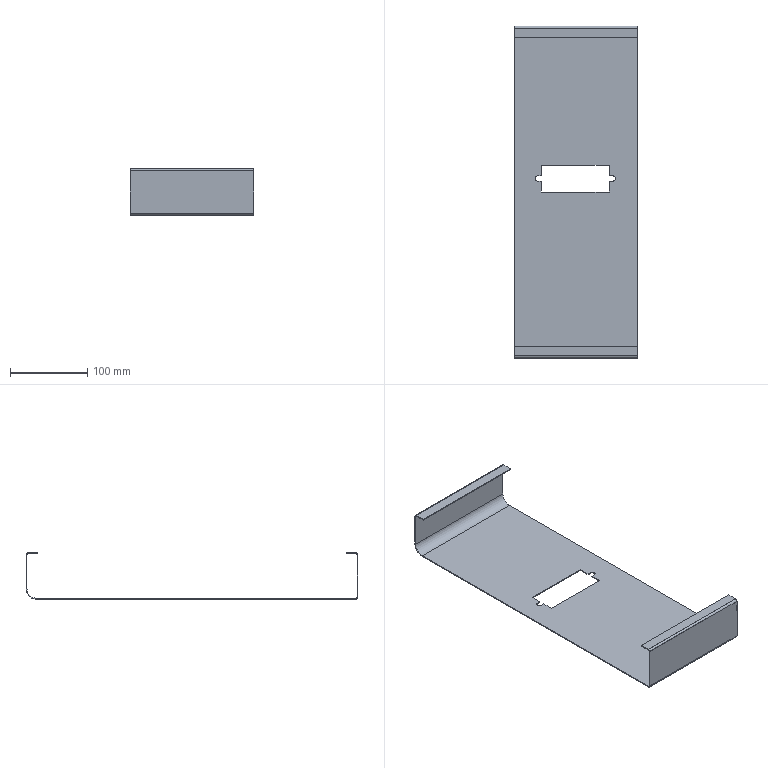Part | SolidWorks | features FlatPattern 1, ICE 1, SMBaseFlange 1, SheetMetal 1 | 1 solid | 51 faces | box 160 x 430 x 60 mm | volume 105063 mm3 | plane 40 | cylinder 11 | commonest cylinder face diameters 3 x3 5.4 x3 7 x3 24 x1 26.4 x1
STEP:
#1=CARTESIAN_POINT('',(-49.5,21.,1.2));
#2=VERTEX_POINT('',#1);
#3=CARTESIAN_POINT('',(-53.,17.5,1.2));
#4=VERTEX_POINT('',#3);
#5=CARTESIAN_POINT('',(-49.5,17.5,1.2));
#6=DIRECTION('',(0.,0.,1.));
#7=DIRECTION('',(0.,1.,0.));
#8=AXIS2_PLACEMENT_3D('',#5,#6,#7);
#9=CIRCLE('',#8,3.5);
#10=EDGE_CURVE('',#2,#4,#9,.T.);
#11=ORIENTED_EDGE('',*,*,#10,.T.);
#12=CARTESIAN_POINT('',(-53.,17.5,0.));
#13=VERTEX_POINT('',#12);
#14=CARTESIAN_POINT('',(-53.,17.5,60.001));
#15=DIRECTION('',(0.,0.,-1.));
#16=VECTOR('',#15,1000.);
#17=LINE('',#14,#16);
#18=EDGE_CURVE('',#4,#13,#17,.T.);
#19=ORIENTED_EDGE('',*,*,#18,.T.);
#20=CARTESIAN_POINT('',(-49.5,21.,0.));
#21=VERTEX_POINT('',#20);
#22=CARTESIAN_POINT('',(-49.5,17.5,0.));
#23=DIRECTION('',(0.,0.,-1.));
#24=DIRECTION('',(-1.,0.,0.));
#25=AXIS2_PLACEMENT_3D('',#22,#23,#24);
#26=CIRCLE('',#25,3.5);
#27=EDGE_CURVE('',#13,#21,#26,.T.);
#28=ORIENTED_EDGE('',*,*,#27,.T.);
#29=CARTESIAN_POINT('',(-49.5,21.,60.001));
#30=DIRECTION('',(0.,0.,-1.));
#31=VECTOR('',#30,1000.);
#32=LINE('',#29,#31);
#33=EDGE_CURVE('',#2,#21,#32,.T.);
#34=ORIENTED_EDGE('',*,*,#33,.F.);
#35=EDGE_LOOP('',(#11,#19,#28,#34));
#36=FACE_OUTER_BOUND('',#35,.T.);
#37=CARTESIAN_POINT('',(-49.5,17.5,60.001));
#38=DIRECTION('',(0.,0.,-1.));
#39=DIRECTION('',(-1.,0.,0.));
#40=AXIS2_PLACEMENT_3D('',#37,#38,#39);
#41=CYLINDRICAL_SURFACE('',#40,3.5);
#42=ADVANCED_FACE('',(#36),#41,.F.);
#43=CARTESIAN_POINT('',(80.,201.8,0.));
#44=VERTEX_POINT('',#43);
#45=CARTESIAN_POINT('',(80.,201.8,1.2));
#46=VERTEX_POINT('',#45);
#47=CARTESIAN_POINT('',(80.,201.8,0.));
#48=DIRECTION('',(0.,0.,1.));
#49=VECTOR('',#48,1000.);
#50=LINE('',#47,#49);
#51=EDGE_CURVE('',#44,#46,#50,.T.);
#52=ORIENTED_EDGE('',*,*,#51,.F.);
#53=CARTESIAN_POINT('',(80.,215.,13.2));
#54=VERTEX_POINT('',#53);
#55=CARTESIAN_POINT('',(80.,201.8,13.2));
#56=DIRECTION('',(-1.,0.,0.));
#57=DIRECTION('',(0.,0.,-1.));
#58=AXIS2_PLACEMENT_3D('',#55,#56,#57);
#59=CIRCLE('',#58,13.2);
#60=EDGE_CURVE('',#54,#44,#59,.T.);
#61=ORIENTED_EDGE('',*,*,#60,.F.);
#62=CARTESIAN_POINT('',(80.,213.8,13.2));
#63=VERTEX_POINT('',#62);
#64=CARTESIAN_POINT('',(80.,213.8,13.2));
#65=DIRECTION('',(0.,1.,0.));
#66=VECTOR('',#65,1000.);
#67=LINE('',#64,#66);
#68=EDGE_CURVE('',#63,#54,#67,.T.);
#69=ORIENTED_EDGE('',*,*,#68,.F.);
#70=CARTESIAN_POINT('',(80.,201.8,13.2));
#71=DIRECTION('',(-1.,0.,0.));
#72=DIRECTION('',(0.,0.,-1.));
#73=AXIS2_PLACEMENT_3D('',#70,#71,#72);
#74=CIRCLE('',#73,12.);
#75=EDGE_CURVE('',#63,#46,#74,.T.);
#76=ORIENTED_EDGE('',*,*,#75,.T.);
#77=EDGE_LOOP('',(#52,#61,#69,#76));
#78=FACE_OUTER_BOUND('',#77,.T.);
#79=CARTESIAN_POINT('',(80.,201.8,0.));
#80=DIRECTION('',(1.,0.,0.));
#81=DIRECTION('',(0.,0.,-1.));
#82=AXIS2_PLACEMENT_3D('',#79,#80,#81);
#83=PLANE('',#82);
#84=ADVANCED_FACE('',(#78),#83,.T.);
#85=CARTESIAN_POINT('',(80.,-212.3,0.));
#86=VERTEX_POINT('',#85);
#87=CARTESIAN_POINT('',(80.,0.,0.));
#88=DIRECTION('',(0.,-1.,0.));
#89=VECTOR('',#88,1000.);
#90=LINE('',#87,#89);
#91=EDGE_CURVE('',#44,#86,#90,.T.);
#92=ORIENTED_EDGE('',*,*,#91,.F.);
#93=ORIENTED_EDGE('',*,*,#51,.T.);
#94=CARTESIAN_POINT('',(80.,-212.3,1.2));
#95=VERTEX_POINT('',#94);
#96=CARTESIAN_POINT('',(80.,0.,1.2));
#97=DIRECTION('',(0.,-1.,0.));
#98=VECTOR('',#97,1000.);
#99=LINE('',#96,#98);
#100=EDGE_CURVE('',#46,#95,#99,.T.);
#101=ORIENTED_EDGE('',*,*,#100,.T.);
#102=CARTESIAN_POINT('',(80.,-212.3,1.2));
#103=DIRECTION('',(0.,0.,-1.));
#104=VECTOR('',#103,1000.);
#105=LINE('',#102,#104);
#106=EDGE_CURVE('',#95,#86,#105,.T.);
#107=ORIENTED_EDGE('',*,*,#106,.T.);
#108=EDGE_LOOP('',(#92,#93,#101,#107));
#109=FACE_OUTER_BOUND('',#108,.T.);
#110=CARTESIAN_POINT('',(80.,213.8,13.2));
#111=DIRECTION('',(1.,0.,0.));
#112=DIRECTION('',(0.,0.,-1.));
#113=AXIS2_PLACEMENT_3D('',#110,#111,#112);
#114=PLANE('',#113);
#115=ADVANCED_FACE('',(#109),#114,.T.);
#116=CARTESIAN_POINT('',(-80.,215.,13.2));
#117=VERTEX_POINT('',#116);
#118=CARTESIAN_POINT('',(-80.,213.8,13.2));
#119=VERTEX_POINT('',#118);
#120=CARTESIAN_POINT('',(-80.,215.,13.2));
#121=DIRECTION('',(0.,-1.,0.));
#122=VECTOR('',#121,1000.);
#123=LINE('',#120,#122);
#124=EDGE_CURVE('',#117,#119,#123,.T.);
#125=ORIENTED_EDGE('',*,*,#124,.F.);
#126=CARTESIAN_POINT('',(-80.,201.8,0.));
#127=VERTEX_POINT('',#126);
#128=CARTESIAN_POINT('',(-80.,201.8,13.2));
#129=DIRECTION('',(-1.,0.,0.));
#130=DIRECTION('',(0.,0.,-1.));
#131=AXIS2_PLACEMENT_3D('',#128,#129,#130);
#132=CIRCLE('',#131,13.2);
#133=EDGE_CURVE('',#117,#127,#132,.T.);
#134=ORIENTED_EDGE('',*,*,#133,.T.);
#135=CARTESIAN_POINT('',(-80.,201.8,1.2));
#136=VERTEX_POINT('',#135);
#137=CARTESIAN_POINT('',(-80.,201.8,1.2));
#138=DIRECTION('',(0.,0.,-1.));
#139=VECTOR('',#138,1000.);
#140=LINE('',#137,#139);
#141=EDGE_CURVE('',#136,#127,#140,.T.);
#142=ORIENTED_EDGE('',*,*,#141,.F.);
#143=CARTESIAN_POINT('',(-80.,201.8,13.2));
#144=DIRECTION('',(-1.,0.,0.));
#145=DIRECTION('',(0.,0.,-1.));
#146=AXIS2_PLACEMENT_3D('',#143,#144,#145);
#147=CIRCLE('',#146,12.);
#148=EDGE_CURVE('',#119,#136,#147,.T.);
#149=ORIENTED_EDGE('',*,*,#148,.F.);
#150=EDGE_LOOP('',(#125,#134,#142,#149));
#151=FACE_OUTER_BOUND('',#150,.T.);
#152=CARTESIAN_POINT('',(-80.,215.,13.2));
#153=DIRECTION('',(-1.,0.,0.));
#154=DIRECTION('',(0.,0.,1.));
#155=AXIS2_PLACEMENT_3D('',#152,#153,#154);
#156=PLANE('',#155);
#157=ADVANCED_FACE('',(#151),#156,.T.);
#158=CARTESIAN_POINT('',(-80.,215.,57.3));
#159=VERTEX_POINT('',#158);
#160=CARTESIAN_POINT('',(-80.,215.,13.2));
#161=DIRECTION('',(0.,0.,-1.));
#162=VECTOR('',#161,1000.);
#163=LINE('',#160,#162);
#164=EDGE_CURVE('',#159,#117,#163,.T.);
#165=ORIENTED_EDGE('',*,*,#164,.T.);
#166=ORIENTED_EDGE('',*,*,#124,.T.);
#167=CARTESIAN_POINT('',(-80.,213.8,57.3));
#168=VERTEX_POINT('',#167);
#169=CARTESIAN_POINT('',(-80.,213.8,13.2));
#170=DIRECTION('',(0.,0.,-1.));
#171=VECTOR('',#170,1000.);
#172=LINE('',#169,#171);
#173=EDGE_CURVE('',#168,#119,#172,.T.);
#174=ORIENTED_EDGE('',*,*,#173,.F.);
#175=CARTESIAN_POINT('',(-80.,213.8,57.3));
#176=DIRECTION('',(0.,1.,0.));
#177=VECTOR('',#176,1000.);
#178=LINE('',#175,#177);
#179=EDGE_CURVE('',#168,#159,#178,.T.);
#180=ORIENTED_EDGE('',*,*,#179,.T.);
#181=EDGE_LOOP('',(#165,#166,#174,#180));
#182=FACE_OUTER_BOUND('',#181,.T.);
#183=CARTESIAN_POINT('',(-80.,201.8,1.2));
#184=DIRECTION('',(-1.,0.,0.));
#185=DIRECTION('',(0.,0.,1.));
#186=AXIS2_PLACEMENT_3D('',#183,#184,#185);
#187=PLANE('',#186);
#188=ADVANCED_FACE('',(#182),#187,.T.);
#189=CARTESIAN_POINT('',(80.,215.,57.3));
#190=VERTEX_POINT('',#189);
#191=CARTESIAN_POINT('',(80.,213.8,57.3));
#192=VERTEX_POINT('',#191);
#193=CARTESIAN_POINT('',(80.,215.,57.3));
#194=DIRECTION('',(0.,-1.,0.));
#195=VECTOR('',#194,1000.);
#196=LINE('',#193,#195);
#197=EDGE_CURVE('',#190,#192,#196,.T.);
#198=ORIENTED_EDGE('',*,*,#197,.F.);
#199=CARTESIAN_POINT('',(80.,212.3,60.));
#200=VERTEX_POINT('',#199);
#201=CARTESIAN_POINT('',(80.,212.3,57.3));
#202=DIRECTION('',(-1.,0.,0.));
#203=DIRECTION('',(0.,0.,-1.));
#204=AXIS2_PLACEMENT_3D('',#201,#202,#203);
#205=CIRCLE('',#204,2.7);
#206=EDGE_CURVE('',#200,#190,#205,.T.);
#207=ORIENTED_EDGE('',*,*,#206,.F.);
#208=CARTESIAN_POINT('',(80.,212.3,58.8));
#209=VERTEX_POINT('',#208);
#210=CARTESIAN_POINT('',(80.,212.3,58.8));
#211=DIRECTION('',(0.,0.,1.));
#212=VECTOR('',#211,1000.);
#213=LINE('',#210,#212);
#214=EDGE_CURVE('',#209,#200,#213,.T.);
#215=ORIENTED_EDGE('',*,*,#214,.F.);
#216=CARTESIAN_POINT('',(80.,212.3,57.3));
#217=DIRECTION('',(-1.,0.,0.));
#218=DIRECTION('',(0.,0.,-1.));
#219=AXIS2_PLACEMENT_3D('',#216,#217,#218);
#220=CIRCLE('',#219,1.5);
#221=EDGE_CURVE('',#209,#192,#220,.T.);
#222=ORIENTED_EDGE('',*,*,#221,.T.);
#223=EDGE_LOOP('',(#198,#207,#215,#222));
#224=FACE_OUTER_BOUND('',#223,.T.);
#225=CARTESIAN_POINT('',(80.,215.,57.3));
#226=DIRECTION('',(1.,0.,0.));
#227=DIRECTION('',(0.,0.,-1.));
#228=AXIS2_PLACEMENT_3D('',#225,#226,#227);
#229=PLANE('',#228);
#230=ADVANCED_FACE('',(#224),#229,.T.);
#231=CARTESIAN_POINT('',(80.,215.,13.2));
#232=DIRECTION('',(0.,0.,-1.));
#233=VECTOR('',#232,1000.);
#234=LINE('',#231,#233);
#235=EDGE_CURVE('',#190,#54,#234,.T.);
#236=ORIENTED_EDGE('',*,*,#235,.F.);
#237=ORIENTED_EDGE('',*,*,#197,.T.);
#238=CARTESIAN_POINT('',(80.,213.8,13.2));
#239=DIRECTION('',(0.,0.,-1.));
#240=VECTOR('',#239,1000.);
#241=LINE('',#238,#240);
#242=EDGE_CURVE('',#192,#63,#241,.T.);
#243=ORIENTED_EDGE('',*,*,#242,.T.);
#244=ORIENTED_EDGE('',*,*,#68,.T.);
#245=EDGE_LOOP('',(#236,#237,#243,#244));
#246=FACE_OUTER_BOUND('',#245,.T.);
#247=CARTESIAN_POINT('',(80.,212.3,58.8));
#248=DIRECTION('',(1.,0.,0.));
#249=DIRECTION('',(0.,0.,-1.));
#250=AXIS2_PLACEMENT_3D('',#247,#248,#249);
#251=PLANE('',#250);
#252=ADVANCED_FACE('',(#246),#251,.T.);
#253=CARTESIAN_POINT('',(-80.,212.3,60.));
#254=VERTEX_POINT('',#253);
#255=CARTESIAN_POINT('',(-80.,212.3,58.8));
#256=VERTEX_POINT('',#255);
#257=CARTESIAN_POINT('',(-80.,212.3,60.));
#258=DIRECTION('',(0.,0.,-1.));
#259=VECTOR('',#258,1000.);
#260=LINE('',#257,#259);
#261=EDGE_CURVE('',#254,#256,#260,.T.);
#262=ORIENTED_EDGE('',*,*,#261,.F.);
#263=CARTESIAN_POINT('',(-80.,212.3,57.3));
#264=DIRECTION('',(-1.,0.,0.));
#265=DIRECTION('',(0.,0.,-1.));
#266=AXIS2_PLACEMENT_3D('',#263,#264,#265);
#267=CIRCLE('',#266,2.7);
#268=EDGE_CURVE('',#254,#159,#267,.T.);
#269=ORIENTED_EDGE('',*,*,#268,.T.);
#270=ORIENTED_EDGE('',*,*,#179,.F.);
#271=CARTESIAN_POINT('',(-80.,212.3,57.3));
#272=DIRECTION('',(-1.,0.,0.));
#273=DIRECTION('',(0.,0.,-1.));
#274=AXIS2_PLACEMENT_3D('',#271,#272,#273);
#275=CIRCLE('',#274,1.5);
#276=EDGE_CURVE('',#256,#168,#275,.T.);
#277=ORIENTED_EDGE('',*,*,#276,.F.);
#278=EDGE_LOOP('',(#262,#269,#270,#277));
#279=FACE_OUTER_BOUND('',#278,.T.);
#280=CARTESIAN_POINT('',(-80.,212.3,60.));
#281=DIRECTION('',(-1.,0.,0.));
#282=DIRECTION('',(0.,0.,1.));
#283=AXIS2_PLACEMENT_3D('',#280,#281,#282);
#284=PLANE('',#283);
#285=ADVANCED_FACE('',(#279),#284,.T.);
#286=CARTESIAN_POINT('',(-80.,200.,60.));
#287=VERTEX_POINT('',#286);
#288=CARTESIAN_POINT('',(-80.,215.,60.));
#289=DIRECTION('',(0.,1.,0.));
#290=VECTOR('',#289,1000.);
#291=LINE('',#288,#290);
#292=EDGE_CURVE('',#287,#254,#291,.T.);
#293=ORIENTED_EDGE('',*,*,#292,.T.);
#294=ORIENTED_EDGE('',*,*,#261,.T.);
#295=CARTESIAN_POINT('',(-80.,200.,58.8));
#296=VERTEX_POINT('',#295);
#297=CARTESIAN_POINT('',(-80.,215.,58.8));
#298=DIRECTION('',(0.,1.,0.));
#299=VECTOR('',#298,1000.);
#300=LINE('',#297,#299);
#301=EDGE_CURVE('',#296,#256,#300,.T.);
#302=ORIENTED_EDGE('',*,*,#301,.F.);
#303=CARTESIAN_POINT('',(-80.,200.,58.8));
#304=DIRECTION('',(0.,0.,1.));
#305=VECTOR('',#304,1000.);
#306=LINE('',#303,#305);
#307=EDGE_CURVE('',#296,#287,#306,.T.);
#308=ORIENTED_EDGE('',*,*,#307,.T.);
#309=EDGE_LOOP('',(#293,#294,#302,#308));
#310=FACE_OUTER_BOUND('',#309,.T.);
#311=CARTESIAN_POINT('',(-80.,213.8,57.3));
#312=DIRECTION('',(-1.,0.,0.));
#313=DIRECTION('',(0.,0.,1.));
#314=AXIS2_PLACEMENT_3D('',#311,#312,#313);
#315=PLANE('',#314);
#316=ADVANCED_FACE('',(#310),#315,.T.);
#317=CARTESIAN_POINT('',(80.,-215.,2.7));
#318=VERTEX_POINT('',#317);
#319=CARTESIAN_POINT('',(80.,-213.8,2.7));
#320=VERTEX_POINT('',#319);
#321=CARTESIAN_POINT('',(80.,-215.,2.7));
#322=DIRECTION('',(0.,1.,0.));
#323=VECTOR('',#322,1000.);
#324=LINE('',#321,#323);
#325=EDGE_CURVE('',#318,#320,#324,.T.);
#326=ORIENTED_EDGE('',*,*,#325,.F.);
#327=CARTESIAN_POINT('',(80.,-212.3,2.7));
#328=DIRECTION('',(-1.,0.,0.));
#329=DIRECTION('',(0.,0.,-1.));
#330=AXIS2_PLACEMENT_3D('',#327,#328,#329);
#331=CIRCLE('',#330,2.7);
#332=EDGE_CURVE('',#86,#318,#331,.T.);
#333=ORIENTED_EDGE('',*,*,#332,.F.);
#334=ORIENTED_EDGE('',*,*,#106,.F.);
#335=CARTESIAN_POINT('',(80.,-212.3,2.7));
#336=DIRECTION('',(-1.,0.,0.));
#337=DIRECTION('',(0.,0.,-1.));
#338=AXIS2_PLACEMENT_3D('',#335,#336,#337);
#339=CIRCLE('',#338,1.5);
#340=EDGE_CURVE('',#95,#320,#339,.T.);
#341=ORIENTED_EDGE('',*,*,#340,.T.);
#342=EDGE_LOOP('',(#326,#333,#334,#341));
#343=FACE_OUTER_BOUND('',#342,.T.);
#344=CARTESIAN_POINT('',(80.,-215.,2.7));
#345=DIRECTION('',(1.,0.,0.));
#346=DIRECTION('',(0.,0.,-1.));
#347=AXIS2_PLACEMENT_3D('',#344,#345,#346);
#348=PLANE('',#347);
#349=ADVANCED_FACE('',(#343),#348,.T.);
#350=CARTESIAN_POINT('',(80.,-215.,57.3));
#351=VERTEX_POINT('',#350);
#352=CARTESIAN_POINT('',(80.,-215.,0.));
#353=DIRECTION('',(0.,0.,1.));
#354=VECTOR('',#353,1000.);
#355=LINE('',#352,#354);
#356=EDGE_CURVE('',#318,#351,#355,.T.);
#357=ORIENTED_EDGE('',*,*,#356,.F.);
#358=ORIENTED_EDGE('',*,*,#325,.T.);
#359=CARTESIAN_POINT('',(80.,-213.8,57.3));
#360=VERTEX_POINT('',#359);
#361=CARTESIAN_POINT('',(80.,-213.8,0.));
#362=DIRECTION('',(0.,0.,1.));
#363=VECTOR('',#362,1000.);
#364=LINE('',#361,#363);
#365=EDGE_CURVE('',#320,#360,#364,.T.);
#366=ORIENTED_EDGE('',*,*,#365,.T.);
#367=CARTESIAN_POINT('',(80.,-213.8,57.3));
#368=DIRECTION('',(0.,-1.,0.));
#369=VECTOR('',#368,1000.);
#370=LINE('',#367,#369);
#371=EDGE_CURVE('',#360,#351,#370,.T.);
#372=ORIENTED_EDGE('',*,*,#371,.T.);
#373=EDGE_LOOP('',(#357,#358,#366,#372));
#374=FACE_OUTER_BOUND('',#373,.T.);
#375=CARTESIAN_POINT('',(80.,-212.3,1.2));
#376=DIRECTION('',(1.,0.,0.));
#377=DIRECTION('',(0.,0.,-1.));
#378=AXIS2_PLACEMENT_3D('',#375,#376,#377);
#379=PLANE('',#378);
#380=ADVANCED_FACE('',(#374),#379,.T.);
#381=CARTESIAN_POINT('',(-80.,-212.3,0.));
#382=VERTEX_POINT('',#381);
#383=CARTESIAN_POINT('',(-80.,-212.3,1.2));
#384=VERTEX_POINT('',#383);
#385=CARTESIAN_POINT('',(-80.,-212.3,0.));
#386=DIRECTION('',(0.,0.,1.));
#387=VECTOR('',#386,1000.);
#388=LINE('',#385,#387);
#389=EDGE_CURVE('',#382,#384,#388,.T.);
#390=ORIENTED_EDGE('',*,*,#389,.F.);
#391=CARTESIAN_POINT('',(-80.,-215.,2.7));
#392=VERTEX_POINT('',#391);
#393=CARTESIAN_POINT('',(-80.,-212.3,2.7));
#394=DIRECTION('',(-1.,0.,0.));
#395=DIRECTION('',(0.,0.,-1.));
#396=AXIS2_PLACEMENT_3D('',#393,#394,#395);
#397=CIRCLE('',#396,2.7);
#398=EDGE_CURVE('',#382,#392,#397,.T.);
#399=ORIENTED_EDGE('',*,*,#398,.T.);
#400=CARTESIAN_POINT('',(-80.,-213.8,2.7));
#401=VERTEX_POINT('',#400);
#402=CARTESIAN_POINT('',(-80.,-213.8,2.7));
#403=DIRECTION('',(0.,-1.,0.));
#404=VECTOR('',#403,1000.);
#405=LINE('',#402,#404);
#406=EDGE_CURVE('',#401,#392,#405,.T.);
#407=ORIENTED_EDGE('',*,*,#406,.F.);
#408=CARTESIAN_POINT('',(-80.,-212.3,2.7));
#409=DIRECTION('',(-1.,0.,0.));
#410=DIRECTION('',(0.,0.,-1.));
#411=AXIS2_PLACEMENT_3D('',#408,#409,#410);
#412=CIRCLE('',#411,1.5);
#413=EDGE_CURVE('',#384,#401,#412,.T.);
#414=ORIENTED_EDGE('',*,*,#413,.F.);
#415=EDGE_LOOP('',(#390,#399,#407,#414));
#416=FACE_OUTER_BOUND('',#415,.T.);
#417=CARTESIAN_POINT('',(-80.,-212.3,0.));
#418=DIRECTION('',(-1.,0.,0.));
#419=DIRECTION('',(0.,0.,1.));
#420=AXIS2_PLACEMENT_3D('',#417,#418,#419);
#421=PLANE('',#420);
#422=ADVANCED_FACE('',(#416),#421,.T.);
#423=CARTESIAN_POINT('',(-80.,0.,0.));
#424=DIRECTION('',(0.,-1.,0.));
#425=VECTOR('',#424,1000.);
#426=LINE('',#423,#425);
#427=EDGE_CURVE('',#127,#382,#426,.T.);
#428=ORIENTED_EDGE('',*,*,#427,.T.);
#429=ORIENTED_EDGE('',*,*,#389,.T.);
#430=CARTESIAN_POINT('',(-80.,0.,1.2));
#431=DIRECTION('',(0.,-1.,0.));
#432=VECTOR('',#431,1000.);
#433=LINE('',#430,#432);
#434=EDGE_CURVE('',#136,#384,#433,.T.);
#435=ORIENTED_EDGE('',*,*,#434,.F.);
#436=ORIENTED_EDGE('',*,*,#141,.T.);
#437=EDGE_LOOP('',(#428,#429,#435,#436));
#438=FACE_OUTER_BOUND('',#437,.T.);
#439=CARTESIAN_POINT('',(-80.,-213.8,2.7));
#440=DIRECTION('',(-1.,0.,0.));
#441=DIRECTION('',(0.,0.,1.));
#442=AXIS2_PLACEMENT_3D('',#439,#440,#441);
#443=PLANE('',#442);
#444=ADVANCED_FACE('',(#438),#443,.T.);
#445=CARTESIAN_POINT('',(80.,-212.3,60.));
#446=VERTEX_POINT('',#445);
#447=CARTESIAN_POINT('',(80.,-212.3,58.8));
#448=VERTEX_POINT('',#447);
#449=CARTESIAN_POINT('',(80.,-212.3,60.));
#450=DIRECTION('',(0.,0.,-1.));
#451=VECTOR('',#450,1000.);
#452=LINE('',#449,#451);
#453=EDGE_CURVE('',#446,#448,#452,.T.);
#454=ORIENTED_EDGE('',*,*,#453,.F.);
#455=CARTESIAN_POINT('',(80.,-212.3,57.3));
#456=DIRECTION('',(-1.,0.,0.));
#457=DIRECTION('',(0.,0.,-1.));
#458=AXIS2_PLACEMENT_3D('',#455,#456,#457);
#459=CIRCLE('',#458,2.7);
#460=EDGE_CURVE('',#351,#446,#459,.T.);
#461=ORIENTED_EDGE('',*,*,#460,.F.);
#462=ORIENTED_EDGE('',*,*,#371,.F.);
#463=CARTESIAN_POINT('',(80.,-212.3,57.3));
#464=DIRECTION('',(-1.,0.,0.));
#465=DIRECTION('',(0.,0.,-1.));
#466=AXIS2_PLACEMENT_3D('',#463,#464,#465);
#467=CIRCLE('',#466,1.5);
#468=EDGE_CURVE('',#360,#448,#467,.T.);
#469=ORIENTED_EDGE('',*,*,#468,.T.);
#470=EDGE_LOOP('',(#454,#461,#462,#469));
#471=FACE_OUTER_BOUND('',#470,.T.);
#472=CARTESIAN_POINT('',(80.,-212.3,60.));
#473=DIRECTION('',(1.,0.,0.));
#474=DIRECTION('',(0.,0.,-1.));
#475=AXIS2_PLACEMENT_3D('',#472,#473,#474);
#476=PLANE('',#475);
#477=ADVANCED_FACE('',(#471),#476,.T.);
#478=CARTESIAN_POINT('',(80.,-200.,60.));
#479=VERTEX_POINT('',#478);
#480=CARTESIAN_POINT('',(80.,-215.,60.));
#481=DIRECTION('',(0.,1.,0.));
#482=VECTOR('',#481,1000.);
#483=LINE('',#480,#482);
#484=EDGE_CURVE('',#446,#479,#483,.T.);
#485=ORIENTED_EDGE('',*,*,#484,.F.);
#486=ORIENTED_EDGE('',*,*,#453,.T.);
#487=CARTESIAN_POINT('',(80.,-200.,58.8));
#488=VERTEX_POINT('',#487);
#489=CARTESIAN_POINT('',(80.,-215.,58.8));
#490=DIRECTION('',(0.,1.,0.));
#491=VECTOR('',#490,1000.);
#492=LINE('',#489,#491);
#493=EDGE_CURVE('',#448,#488,#492,.T.);
#494=ORIENTED_EDGE('',*,*,#493,.T.);
#495=CARTESIAN_POINT('',(80.,-200.,60.));
#496=DIRECTION('',(0.,0.,-1.));
#497=VECTOR('',#496,1000.);
#498=LINE('',#495,#497);
#499=EDGE_CURVE('',#479,#488,#498,.T.);
#500=ORIENTED_EDGE('',*,*,#499,.F.);
#501=EDGE_LOOP('',(#485,#486,#494,#500));
#502=FACE_OUTER_BOUND('',#501,.T.);
#503=CARTESIAN_POINT('',(80.,-213.8,57.3));
#504=DIRECTION('',(1.,0.,0.));
#505=DIRECTION('',(0.,0.,-1.));
#506=AXIS2_PLACEMENT_3D('',#503,#504,#505);
#507=PLANE('',#506);
#508=ADVANCED_FACE('',(#502),#507,.T.);
#509=CARTESIAN_POINT('',(-80.,-215.,57.3));
#510=VERTEX_POINT('',#509);
#511=CARTESIAN_POINT('',(-80.,-213.8,57.3));
#512=VERTEX_POINT('',#511);
#513=CARTESIAN_POINT('',(-80.,-215.,57.3));
#514=DIRECTION('',(0.,1.,0.));
#515=VECTOR('',#514,1000.);
#516=LINE('',#513,#515);
#517=EDGE_CURVE('',#510,#512,#516,.T.);
#518=ORIENTED_EDGE('',*,*,#517,.F.);
#519=CARTESIAN_POINT('',(-80.,-212.3,60.));
#520=VERTEX_POINT('',#519);
#521=CARTESIAN_POINT('',(-80.,-212.3,57.3));
#522=DIRECTION('',(-1.,0.,0.));
#523=DIRECTION('',(0.,0.,-1.));
#524=AXIS2_PLACEMENT_3D('',#521,#522,#523);
#525=CIRCLE('',#524,2.7);
#526=EDGE_CURVE('',#510,#520,#525,.T.);
#527=ORIENTED_EDGE('',*,*,#526,.T.);
#528=CARTESIAN_POINT('',(-80.,-212.3,58.8));
#529=VERTEX_POINT('',#528);
#530=CARTESIAN_POINT('',(-80.,-212.3,58.8));
#531=DIRECTION('',(0.,0.,1.));
#532=VECTOR('',#531,1000.);
#533=LINE('',#530,#532);
#534=EDGE_CURVE('',#529,#520,#533,.T.);
#535=ORIENTED_EDGE('',*,*,#534,.F.);
#536=CARTESIAN_POINT('',(-80.,-212.3,57.3));
#537=DIRECTION('',(-1.,0.,0.));
#538=DIRECTION('',(0.,0.,-1.));
#539=AXIS2_PLACEMENT_3D('',#536,#537,#538);
#540=CIRCLE('',#539,1.5);
#541=EDGE_CURVE('',#512,#529,#540,.T.);
#542=ORIENTED_EDGE('',*,*,#541,.F.);
#543=EDGE_LOOP('',(#518,#527,#535,#542));
#544=FACE_OUTER_BOUND('',#543,.T.);
#545=CARTESIAN_POINT('',(-80.,-215.,57.3));
#546=DIRECTION('',(-1.,0.,0.));
#547=DIRECTION('',(0.,0.,1.));
#548=AXIS2_PLACEMENT_3D('',#545,#546,#547);
#549=PLANE('',#548);
#550=ADVANCED_FACE('',(#544),#549,.T.);
#551=CARTESIAN_POINT('',(-80.,-215.,0.));
#552=DIRECTION('',(0.,0.,1.));
#553=VECTOR('',#552,1000.);
#554=LINE('',#551,#553);
#555=EDGE_CURVE('',#392,#510,#554,.T.);
#556=ORIENTED_EDGE('',*,*,#555,.T.);
#557=ORIENTED_EDGE('',*,*,#517,.T.);
#558=CARTESIAN_POINT('',(-80.,-213.8,0.));
#559=DIRECTION('',(0.,0.,1.));
#560=VECTOR('',#559,1000.);
#561=LINE('',#558,#560);
#562=EDGE_CURVE('',#401,#512,#561,.T.);
#563=ORIENTED_EDGE('',*,*,#562,.F.);
#564=ORIENTED_EDGE('',*,*,#406,.T.);
#565=EDGE_LOOP('',(#556,#557,#563,#564));
#566=FACE_OUTER_BOUND('',#565,.T.);
#567=CARTESIAN_POINT('',(-80.,-212.3,58.8));
#568=DIRECTION('',(-1.,0.,0.));
#569=DIRECTION('',(0.,0.,1.));
#570=AXIS2_PLACEMENT_3D('',#567,#568,#569);
#571=PLANE('',#570);
#572=ADVANCED_FACE('',(#566),#571,.T.);
#573=CARTESIAN_POINT('',(-80.,-200.,58.8));
#574=VERTEX_POINT('',#573);
#575=CARTESIAN_POINT('',(-80.,-215.,58.8));
#576=DIRECTION('',(0.,1.,0.));
#577=VECTOR('',#576,1000.);
#578=LINE('',#575,#577);
#579=EDGE_CURVE('',#529,#574,#578,.T.);
#580=ORIENTED_EDGE('',*,*,#579,.T.);
#581=CARTESIAN_POINT('',(80.,-200.,58.8));
#582=DIRECTION('',(-1.,0.,0.));
#583=VECTOR('',#582,1000.);
#584=LINE('',#581,#583);
#585=EDGE_CURVE('',#488,#574,#584,.T.);
#586=ORIENTED_EDGE('',*,*,#585,.F.);
#587=ORIENTED_EDGE('',*,*,#493,.F.);
#588=CARTESIAN_POINT('',(80.,-212.3,58.8));
#589=DIRECTION('',(-1.,0.,0.));
#590=VECTOR('',#589,1000.);
#591=LINE('',#588,#590);
#592=EDGE_CURVE('',#448,#529,#591,.T.);
#593=ORIENTED_EDGE('',*,*,#592,.T.);
#594=EDGE_LOOP('',(#580,#586,#587,#593));
#595=FACE_OUTER_BOUND('',#594,.T.);
#596=CARTESIAN_POINT('',(80.,-215.,58.8));
#597=DIRECTION('',(0.,0.,1.));
#598=DIRECTION('',(1.,0.,0.));
#599=AXIS2_PLACEMENT_3D('',#596,#597,#598);
#600=PLANE('',#599);
#601=ADVANCED_FACE('',(#595),#600,.F.);
#602=CARTESIAN_POINT('',(-80.,-200.,60.));
#603=VERTEX_POINT('',#602);
#604=CARTESIAN_POINT('',(-80.,-200.,60.));
#605=DIRECTION('',(0.,0.,-1.));
#606=VECTOR('',#605,1000.);
#607=LINE('',#604,#606);
#608=EDGE_CURVE('',#603,#574,#607,.T.);
#609=ORIENTED_EDGE('',*,*,#608,.F.);
#610=CARTESIAN_POINT('',(80.,-200.,60.));
#611=DIRECTION('',(-1.,0.,0.));
#612=VECTOR('',#611,1000.);
#613=LINE('',#610,#612);
#614=EDGE_CURVE('',#479,#603,#613,.T.);
#615=ORIENTED_EDGE('',*,*,#614,.F.);
#616=ORIENTED_EDGE('',*,*,#499,.T.);
#617=ORIENTED_EDGE('',*,*,#585,.T.);
#618=EDGE_LOOP('',(#609,#615,#616,#617));
#619=FACE_OUTER_BOUND('',#618,.T.);
#620=CARTESIAN_POINT('',(80.,-200.,60.));
#621=DIRECTION('',(0.,1.,0.));
#622=DIRECTION('',(0.,0.,1.));
#623=AXIS2_PLACEMENT_3D('',#620,#621,#622);
#624=PLANE('',#623);
#625=ADVANCED_FACE('',(#619),#624,.T.);
#626=CARTESIAN_POINT('',(-80.,-215.,60.));
#627=DIRECTION('',(0.,1.,0.));
#628=VECTOR('',#627,1000.);
#629=LINE('',#626,#628);
#630=EDGE_CURVE('',#520,#603,#629,.T.);
#631=ORIENTED_EDGE('',*,*,#630,.F.);
#632=CARTESIAN_POINT('',(80.,-212.3,60.));
#633=DIRECTION('',(-1.,0.,0.));
#634=VECTOR('',#633,1000.);
#635=LINE('',#632,#634);
#636=EDGE_CURVE('',#446,#520,#635,.T.);
#637=ORIENTED_EDGE('',*,*,#636,.F.);
#638=ORIENTED_EDGE('',*,*,#484,.T.);
#639=ORIENTED_EDGE('',*,*,#614,.T.);
#640=EDGE_LOOP('',(#631,#637,#638,#639));
#641=FACE_OUTER_BOUND('',#640,.T.);
#642=CARTESIAN_POINT('',(80.,-215.,60.));
#643=DIRECTION('',(0.,0.,1.));
#644=DIRECTION('',(1.,0.,0.));
#645=AXIS2_PLACEMENT_3D('',#642,#643,#644);
#646=PLANE('',#645);
#647=ADVANCED_FACE('',(#641),#646,.T.);
#648=ORIENTED_EDGE('',*,*,#526,.F.);
#649=CARTESIAN_POINT('',(80.,-215.,57.3));
#650=DIRECTION('',(-1.,0.,0.));
#651=VECTOR('',#650,1000.);
#652=LINE('',#649,#651);
#653=EDGE_CURVE('',#351,#510,#652,.T.);
#654=ORIENTED_EDGE('',*,*,#653,.F.);
#655=ORIENTED_EDGE('',*,*,#460,.T.);
#656=ORIENTED_EDGE('',*,*,#636,.T.);
#657=EDGE_LOOP('',(#648,#654,#655,#656));
#658=FACE_OUTER_BOUND('',#657,.T.);
#659=CARTESIAN_POINT('',(80.,-212.3,57.3));
#660=DIRECTION('',(-1.,0.,0.));
#661=DIRECTION('',(0.,0.,1.));
#662=AXIS2_PLACEMENT_3D('',#659,#660,#661);
#663=CYLINDRICAL_SURFACE('',#662,2.7);
#664=ADVANCED_FACE('',(#658),#663,.T.);
#665=ORIENTED_EDGE('',*,*,#555,.F.);
#666=CARTESIAN_POINT('',(80.,-215.,2.7));
#667=DIRECTION('',(-1.,0.,0.));
#668=VECTOR('',#667,1000.);
#669=LINE('',#666,#668);
#670=EDGE_CURVE('',#318,#392,#669,.T.);
#671=ORIENTED_EDGE('',*,*,#670,.F.);
#672=ORIENTED_EDGE('',*,*,#356,.T.);
#673=ORIENTED_EDGE('',*,*,#653,.T.);
#674=EDGE_LOOP('',(#665,#671,#672,#673));
#675=FACE_OUTER_BOUND('',#674,.T.);
#676=CARTESIAN_POINT('',(80.,-215.,0.));
#677=DIRECTION('',(0.,-1.,0.));
#678=DIRECTION('',(0.,0.,-1.));
#679=AXIS2_PLACEMENT_3D('',#676,#677,#678);
#680=PLANE('',#679);
#681=ADVANCED_FACE('',(#675),#680,.T.);
#682=ORIENTED_EDGE('',*,*,#398,.F.);
#683=CARTESIAN_POINT('',(80.,-212.3,0.));
#684=DIRECTION('',(-1.,0.,0.));
#685=VECTOR('',#684,1000.);
#686=LINE('',#683,#685);
#687=EDGE_CURVE('',#86,#382,#686,.T.);
#688=ORIENTED_EDGE('',*,*,#687,.F.);
#689=ORIENTED_EDGE('',*,*,#332,.T.);
#690=ORIENTED_EDGE('',*,*,#670,.T.);
#691=EDGE_LOOP('',(#682,#688,#689,#690));
#692=FACE_OUTER_BOUND('',#691,.T.);
#693=CARTESIAN_POINT('',(80.,-212.3,2.7));
#694=DIRECTION('',(-1.,0.,0.));
#695=DIRECTION('',(0.,0.,1.));
#696=AXIS2_PLACEMENT_3D('',#693,#694,#695);
#697=CYLINDRICAL_SURFACE('',#696,2.7);
#698=ADVANCED_FACE('',(#692),#697,.T.);
#699=CARTESIAN_POINT('',(43.,35.,0.));
#700=VERTEX_POINT('',#699);
#701=CARTESIAN_POINT('',(43.,21.,0.));
#702=VERTEX_POINT('',#701);
#703=CARTESIAN_POINT('',(43.,35.,0.));
#704=DIRECTION('',(0.,-1.,0.));
#705=VECTOR('',#704,1000.);
#706=LINE('',#703,#705);
#707=EDGE_CURVE('',#700,#702,#706,.T.);
#708=ORIENTED_EDGE('',*,*,#707,.F.);
#709=CARTESIAN_POINT('',(-45.,35.,0.));
#710=VERTEX_POINT('',#709);
#711=CARTESIAN_POINT('',(43.,35.,0.));
#712=DIRECTION('',(1.,0.,0.));
#713=VECTOR('',#712,1000.);
#714=LINE('',#711,#713);
#715=EDGE_CURVE('',#710,#700,#714,.T.);
#716=ORIENTED_EDGE('',*,*,#715,.F.);
#717=CARTESIAN_POINT('',(-45.,21.,0.));
#718=VERTEX_POINT('',#717);
#719=CARTESIAN_POINT('',(-45.,35.,0.));
#720=DIRECTION('',(0.,1.,0.));
#721=VECTOR('',#720,1000.);
#722=LINE('',#719,#721);
#723=EDGE_CURVE('',#718,#710,#722,.T.);
#724=ORIENTED_EDGE('',*,*,#723,.F.);
#725=CARTESIAN_POINT('',(-49.5,21.,0.));
#726=DIRECTION('',(1.,0.,0.));
#727=VECTOR('',#726,1000.);
#728=LINE('',#725,#727);
#729=EDGE_CURVE('',#21,#718,#728,.T.);
#730=ORIENTED_EDGE('',*,*,#729,.F.);
#731=ORIENTED_EDGE('',*,*,#27,.F.);
#732=CARTESIAN_POINT('',(-49.5,14.,0.));
#733=VERTEX_POINT('',#732);
#734=CARTESIAN_POINT('',(-49.5,17.5,0.));
#735=DIRECTION('',(0.,0.,-1.));
#736=DIRECTION('',(-1.,0.,0.));
#737=AXIS2_PLACEMENT_3D('',#734,#735,#736);
#738=CIRCLE('',#737,3.5);
#739=EDGE_CURVE('',#733,#13,#738,.T.);
#740=ORIENTED_EDGE('',*,*,#739,.F.);
#741=CARTESIAN_POINT('',(-45.,14.,0.));
#742=VERTEX_POINT('',#741);
#743=CARTESIAN_POINT('',(-49.5,14.,0.));
#744=DIRECTION('',(-1.,0.,0.));
#745=VECTOR('',#744,1000.);
#746=LINE('',#743,#745);
#747=EDGE_CURVE('',#742,#733,#746,.T.);
#748=ORIENTED_EDGE('',*,*,#747,.F.);
#749=CARTESIAN_POINT('',(-45.,0.,0.));
#750=VERTEX_POINT('',#749);
#751=CARTESIAN_POINT('',(-45.,14.,0.));
#752=DIRECTION('',(0.,1.,0.));
#753=VECTOR('',#752,1000.);
#754=LINE('',#751,#753);
#755=EDGE_CURVE('',#750,#742,#754,.T.);
#756=ORIENTED_EDGE('',*,*,#755,.F.);
#757=CARTESIAN_POINT('',(43.,0.,0.));
#758=VERTEX_POINT('',#757);
#759=CARTESIAN_POINT('',(43.,0.,0.));
#760=DIRECTION('',(-1.,0.,0.));
#761=VECTOR('',#760,1000.);
#762=LINE('',#759,#761);
#763=EDGE_CURVE('',#758,#750,#762,.T.);
#764=ORIENTED_EDGE('',*,*,#763,.F.);
#765=CARTESIAN_POINT('',(43.,14.,0.));
#766=VERTEX_POINT('',#765);
#767=CARTESIAN_POINT('',(43.,14.,0.));
#768=DIRECTION('',(0.,-1.,0.));
#769=VECTOR('',#768,1000.);
#770=LINE('',#767,#769);
#771=EDGE_CURVE('',#766,#758,#770,.T.);
#772=ORIENTED_EDGE('',*,*,#771,.F.);
#773=CARTESIAN_POINT('',(47.5,14.,0.));
#774=VERTEX_POINT('',#773);
#775=CARTESIAN_POINT('',(47.5,14.,0.));
#776=DIRECTION('',(-1.,0.,0.));
#777=VECTOR('',#776,1000.);
#778=LINE('',#775,#777);
#779=EDGE_CURVE('',#774,#766,#778,.T.);
#780=ORIENTED_EDGE('',*,*,#779,.F.);
#781=CARTESIAN_POINT('',(47.5,21.,0.));
#782=VERTEX_POINT('',#781);
#783=CARTESIAN_POINT('',(47.5,17.5,0.));
#784=DIRECTION('',(0.,0.,-1.));
#785=DIRECTION('',(1.,0.,0.));
#786=AXIS2_PLACEMENT_3D('',#783,#784,#785);
#787=CIRCLE('',#786,3.5);
#788=EDGE_CURVE('',#782,#774,#787,.T.);
#789=ORIENTED_EDGE('',*,*,#788,.F.);
#790=CARTESIAN_POINT('',(47.5,21.,0.));
#791=DIRECTION('',(1.,0.,0.));
#792=VECTOR('',#791,1000.);
#793=LINE('',#790,#792);
#794=EDGE_CURVE('',#702,#782,#793,.T.);
#795=ORIENTED_EDGE('',*,*,#794,.F.);
#796=EDGE_LOOP('',(#708,#716,#724,#730,#731,#740,#748,#756,#764,#772,#780,#789,#795));
#797=FACE_BOUND('',#796,.T.);
#798=ORIENTED_EDGE('',*,*,#427,.F.);
#799=CARTESIAN_POINT('',(80.,201.8,0.));
#800=DIRECTION('',(-1.,0.,0.));
#801=VECTOR('',#800,1000.);
#802=LINE('',#799,#801);
#803=EDGE_CURVE('',#44,#127,#802,.T.);
#804=ORIENTED_EDGE('',*,*,#803,.F.);
#805=ORIENTED_EDGE('',*,*,#91,.T.);
#806=ORIENTED_EDGE('',*,*,#687,.T.);
#807=EDGE_LOOP('',(#798,#804,#805,#806));
#808=FACE_OUTER_BOUND('',#807,.T.);
#809=CARTESIAN_POINT('',(80.,0.,0.));
#810=DIRECTION('',(0.,0.,-1.));
#811=DIRECTION('',(0.,1.,0.));
#812=AXIS2_PLACEMENT_3D('',#809,#810,#811);
#813=PLANE('',#812);
#814=ADVANCED_FACE('',(#797,#808),#813,.T.);
#815=ORIENTED_EDGE('',*,*,#133,.F.);
#816=CARTESIAN_POINT('',(80.,215.,13.2));
#817=DIRECTION('',(-1.,0.,0.));
#818=VECTOR('',#817,1000.);
#819=LINE('',#816,#818);
#820=EDGE_CURVE('',#54,#117,#819,.T.);
#821=ORIENTED_EDGE('',*,*,#820,.F.);
#822=ORIENTED_EDGE('',*,*,#60,.T.);
#823=ORIENTED_EDGE('',*,*,#803,.T.);
#824=EDGE_LOOP('',(#815,#821,#822,#823));
#825=FACE_OUTER_BOUND('',#824,.T.);
#826=CARTESIAN_POINT('',(80.,201.8,13.2));
#827=DIRECTION('',(-1.,0.,0.));
#828=DIRECTION('',(0.,0.,1.));
#829=AXIS2_PLACEMENT_3D('',#826,#827,#828);
#830=CYLINDRICAL_SURFACE('',#829,13.2);
#831=ADVANCED_FACE('',(#825),#830,.T.);
#832=ORIENTED_EDGE('',*,*,#164,.F.);
#833=CARTESIAN_POINT('',(80.,215.,57.3));
#834=DIRECTION('',(-1.,0.,0.));
#835=VECTOR('',#834,1000.);
#836=LINE('',#833,#835);
#837=EDGE_CURVE('',#190,#159,#836,.T.);
#838=ORIENTED_EDGE('',*,*,#837,.F.);
#839=ORIENTED_EDGE('',*,*,#235,.T.);
#840=ORIENTED_EDGE('',*,*,#820,.T.);
#841=EDGE_LOOP('',(#832,#838,#839,#840));
#842=FACE_OUTER_BOUND('',#841,.T.);
#843=CARTESIAN_POINT('',(80.,215.,13.2));
#844=DIRECTION('',(0.,1.,0.));
#845=DIRECTION('',(0.,0.,1.));
#846=AXIS2_PLACEMENT_3D('',#843,#844,#845);
#847=PLANE('',#846);
#848=ADVANCED_FACE('',(#842),#847,.T.);
#849=ORIENTED_EDGE('',*,*,#268,.F.);
#850=CARTESIAN_POINT('',(80.,212.3,60.));
#851=DIRECTION('',(-1.,0.,0.));
#852=VECTOR('',#851,1000.);
#853=LINE('',#850,#852);
#854=EDGE_CURVE('',#200,#254,#853,.T.);
#855=ORIENTED_EDGE('',*,*,#854,.F.);
#856=ORIENTED_EDGE('',*,*,#206,.T.);
#857=ORIENTED_EDGE('',*,*,#837,.T.);
#858=EDGE_LOOP('',(#849,#855,#856,#857));
#859=FACE_OUTER_BOUND('',#858,.T.);
#860=CARTESIAN_POINT('',(80.,212.3,57.3));
#861=DIRECTION('',(-1.,0.,0.));
#862=DIRECTION('',(0.,0.,1.));
#863=AXIS2_PLACEMENT_3D('',#860,#861,#862);
#864=CYLINDRICAL_SURFACE('',#863,2.7);
#865=ADVANCED_FACE('',(#859),#864,.T.);
#866=ORIENTED_EDGE('',*,*,#292,.F.);
#867=CARTESIAN_POINT('',(80.,200.,60.));
#868=VERTEX_POINT('',#867);
#869=CARTESIAN_POINT('',(80.,200.,60.));
#870=DIRECTION('',(-1.,0.,0.));
#871=VECTOR('',#870,1000.);
#872=LINE('',#869,#871);
#873=EDGE_CURVE('',#868,#287,#872,.T.);
#874=ORIENTED_EDGE('',*,*,#873,.F.);
#875=CARTESIAN_POINT('',(80.,215.,60.));
#876=DIRECTION('',(0.,1.,0.));
#877=VECTOR('',#876,1000.);
#878=LINE('',#875,#877);
#879=EDGE_CURVE('',#868,#200,#878,.T.);
#880=ORIENTED_EDGE('',*,*,#879,.T.);
#881=ORIENTED_EDGE('',*,*,#854,.T.);
#882=EDGE_LOOP('',(#866,#874,#880,#881));
#883=FACE_OUTER_BOUND('',#882,.T.);
#884=CARTESIAN_POINT('',(80.,215.,60.));
#885=DIRECTION('',(0.,0.,1.));
#886=DIRECTION('',(0.,-1.,0.));
#887=AXIS2_PLACEMENT_3D('',#884,#885,#886);
#888=PLANE('',#887);
#889=ADVANCED_FACE('',(#883),#888,.T.);
#890=ORIENTED_EDGE('',*,*,#307,.F.);
#891=CARTESIAN_POINT('',(80.,200.,58.8));
#892=VERTEX_POINT('',#891);
#893=CARTESIAN_POINT('',(80.,200.,58.8));
#894=DIRECTION('',(-1.,0.,0.));
#895=VECTOR('',#894,1000.);
#896=LINE('',#893,#895);
#897=EDGE_CURVE('',#892,#296,#896,.T.);
#898=ORIENTED_EDGE('',*,*,#897,.F.);
#899=CARTESIAN_POINT('',(80.,200.,58.8));
#900=DIRECTION('',(0.,0.,1.));
#901=VECTOR('',#900,1000.);
#902=LINE('',#899,#901);
#903=EDGE_CURVE('',#892,#868,#902,.T.);
#904=ORIENTED_EDGE('',*,*,#903,.T.);
#905=ORIENTED_EDGE('',*,*,#873,.T.);
#906=EDGE_LOOP('',(#890,#898,#904,#905));
#907=FACE_OUTER_BOUND('',#906,.T.);
#908=CARTESIAN_POINT('',(80.,200.,58.8));
#909=DIRECTION('',(0.,-1.,0.));
#910=DIRECTION('',(0.,0.,-1.));
#911=AXIS2_PLACEMENT_3D('',#908,#909,#910);
#912=PLANE('',#911);
#913=ADVANCED_FACE('',(#907),#912,.T.);
#914=ORIENTED_EDGE('',*,*,#301,.T.);
#915=CARTESIAN_POINT('',(80.,212.3,58.8));
#916=DIRECTION('',(-1.,0.,0.));
#917=VECTOR('',#916,1000.);
#918=LINE('',#915,#917);
#919=EDGE_CURVE('',#209,#256,#918,.T.);
#920=ORIENTED_EDGE('',*,*,#919,.F.);
#921=CARTESIAN_POINT('',(80.,215.,58.8));
#922=DIRECTION('',(0.,1.,0.));
#923=VECTOR('',#922,1000.);
#924=LINE('',#921,#923);
#925=EDGE_CURVE('',#892,#209,#924,.T.);
#926=ORIENTED_EDGE('',*,*,#925,.F.);
#927=ORIENTED_EDGE('',*,*,#897,.T.);
#928=EDGE_LOOP('',(#914,#920,#926,#927));
#929=FACE_OUTER_BOUND('',#928,.T.);
#930=CARTESIAN_POINT('',(80.,215.,58.8));
#931=DIRECTION('',(0.,0.,1.));
#932=DIRECTION('',(0.,-1.,0.));
#933=AXIS2_PLACEMENT_3D('',#930,#931,#932);
#934=PLANE('',#933);
#935=ADVANCED_FACE('',(#929),#934,.F.);
#936=ORIENTED_EDGE('',*,*,#276,.T.);
#937=CARTESIAN_POINT('',(80.,213.8,57.3));
#938=DIRECTION('',(-1.,0.,0.));
#939=VECTOR('',#938,1000.);
#940=LINE('',#937,#939);
#941=EDGE_CURVE('',#192,#168,#940,.T.);
#942=ORIENTED_EDGE('',*,*,#941,.F.);
#943=ORIENTED_EDGE('',*,*,#221,.F.);
#944=ORIENTED_EDGE('',*,*,#919,.T.);
#945=EDGE_LOOP('',(#936,#942,#943,#944));
#946=FACE_OUTER_BOUND('',#945,.T.);
#947=CARTESIAN_POINT('',(80.,212.3,57.3));
#948=DIRECTION('',(-1.,0.,0.));
#949=DIRECTION('',(0.,0.,1.));
#950=AXIS2_PLACEMENT_3D('',#947,#948,#949);
#951=CYLINDRICAL_SURFACE('',#950,1.5);
#952=ADVANCED_FACE('',(#946),#951,.F.);
#953=ORIENTED_EDGE('',*,*,#173,.T.);
#954=CARTESIAN_POINT('',(80.,213.8,13.2));
#955=DIRECTION('',(-1.,0.,0.));
#956=VECTOR('',#955,1000.);
#957=LINE('',#954,#956);
#958=EDGE_CURVE('',#63,#119,#957,.T.);
#959=ORIENTED_EDGE('',*,*,#958,.F.);
#960=ORIENTED_EDGE('',*,*,#242,.F.);
#961=ORIENTED_EDGE('',*,*,#941,.T.);
#962=EDGE_LOOP('',(#953,#959,#960,#961));
#963=FACE_OUTER_BOUND('',#962,.T.);
#964=CARTESIAN_POINT('',(80.,213.8,13.2));
#965=DIRECTION('',(0.,1.,0.));
#966=DIRECTION('',(0.,0.,1.));
#967=AXIS2_PLACEMENT_3D('',#964,#965,#966);
#968=PLANE('',#967);
#969=ADVANCED_FACE('',(#963),#968,.F.);
#970=ORIENTED_EDGE('',*,*,#148,.T.);
#971=CARTESIAN_POINT('',(80.,201.8,1.2));
#972=DIRECTION('',(-1.,0.,0.));
#973=VECTOR('',#972,1000.);
#974=LINE('',#971,#973);
#975=EDGE_CURVE('',#46,#136,#974,.T.);
#976=ORIENTED_EDGE('',*,*,#975,.F.);
#977=ORIENTED_EDGE('',*,*,#75,.F.);
#978=ORIENTED_EDGE('',*,*,#958,.T.);
#979=EDGE_LOOP('',(#970,#976,#977,#978));
#980=FACE_OUTER_BOUND('',#979,.T.);
#981=CARTESIAN_POINT('',(80.,201.8,13.2));
#982=DIRECTION('',(-1.,0.,0.));
#983=DIRECTION('',(0.,0.,1.));
#984=AXIS2_PLACEMENT_3D('',#981,#982,#983);
#985=CYLINDRICAL_SURFACE('',#984,12.);
#986=ADVANCED_FACE('',(#980),#985,.F.);
#987=CARTESIAN_POINT('',(43.,35.,1.2));
#988=VERTEX_POINT('',#987);
#989=CARTESIAN_POINT('',(-45.,35.,1.2));
#990=VERTEX_POINT('',#989);
#991=CARTESIAN_POINT('',(43.,35.,1.2));
#992=DIRECTION('',(-1.,0.,0.));
#993=VECTOR('',#992,1000.);
#994=LINE('',#991,#993);
#995=EDGE_CURVE('',#988,#990,#994,.T.);
#996=ORIENTED_EDGE('',*,*,#995,.F.);
#997=CARTESIAN_POINT('',(43.,21.,1.2));
#998=VERTEX_POINT('',#997);
#999=CARTESIAN_POINT('',(43.,35.,1.2));
#1000=DIRECTION('',(0.,1.,0.));
#1001=VECTOR('',#1000,1000.);
#1002=LINE('',#999,#1001);
#1003=EDGE_CURVE('',#998,#988,#1002,.T.);
#1004=ORIENTED_EDGE('',*,*,#1003,.F.);
#1005=CARTESIAN_POINT('',(47.5,21.,1.2));
#1006=VERTEX_POINT('',#1005);
#1007=CARTESIAN_POINT('',(47.5,21.,1.2));
#1008=DIRECTION('',(-1.,0.,0.));
#1009=VECTOR('',#1008,1000.);
#1010=LINE('',#1007,#1009);
#1011=EDGE_CURVE('',#1006,#998,#1010,.T.);
#1012=ORIENTED_EDGE('',*,*,#1011,.F.);
#1013=CARTESIAN_POINT('',(47.5,14.,1.2));
#1014=VERTEX_POINT('',#1013);
#1015=CARTESIAN_POINT('',(47.5,17.5,1.2));
#1016=DIRECTION('',(0.,0.,1.));
#1017=DIRECTION('',(0.,1.,0.));
#1018=AXIS2_PLACEMENT_3D('',#1015,#1016,#1017);
#1019=CIRCLE('',#1018,3.5);
#1020=EDGE_CURVE('',#1014,#1006,#1019,.T.);
#1021=ORIENTED_EDGE('',*,*,#1020,.F.);
#1022=CARTESIAN_POINT('',(43.,14.,1.2));
#1023=VERTEX_POINT('',#1022);
#1024=CARTESIAN_POINT('',(47.5,14.,1.2));
#1025=DIRECTION('',(1.,0.,0.));
#1026=VECTOR('',#1025,1000.);
#1027=LINE('',#1024,#1026);
#1028=EDGE_CURVE('',#1023,#1014,#1027,.T.);
#1029=ORIENTED_EDGE('',*,*,#1028,.F.);
#1030=CARTESIAN_POINT('',(43.,0.,1.2));
#1031=VERTEX_POINT('',#1030);
#1032=CARTESIAN_POINT('',(43.,14.,1.2));
#1033=DIRECTION('',(0.,1.,0.));
#1034=VECTOR('',#1033,1000.);
#1035=LINE('',#1032,#1034);
#1036=EDGE_CURVE('',#1031,#1023,#1035,.T.);
#1037=ORIENTED_EDGE('',*,*,#1036,.F.);
#1038=CARTESIAN_POINT('',(-45.,0.,1.2));
#1039=VERTEX_POINT('',#1038);
#1040=CARTESIAN_POINT('',(43.,0.,1.2));
#1041=DIRECTION('',(1.,0.,0.));
#1042=VECTOR('',#1041,1000.);
#1043=LINE('',#1040,#1042);
#1044=EDGE_CURVE('',#1039,#1031,#1043,.T.);
#1045=ORIENTED_EDGE('',*,*,#1044,.F.);
#1046=CARTESIAN_POINT('',(-45.,14.,1.2));
#1047=VERTEX_POINT('',#1046);
#1048=CARTESIAN_POINT('',(-45.,14.,1.2));
#1049=DIRECTION('',(0.,-1.,0.));
#1050=VECTOR('',#1049,1000.);
#1051=LINE('',#1048,#1050);
#1052=EDGE_CURVE('',#1047,#1039,#1051,.T.);
#1053=ORIENTED_EDGE('',*,*,#1052,.F.);
#1054=CARTESIAN_POINT('',(-49.5,14.,1.2));
#1055=VERTEX_POINT('',#1054);
#1056=CARTESIAN_POINT('',(-49.5,14.,1.2));
#1057=DIRECTION('',(1.,0.,0.));
#1058=VECTOR('',#1057,1000.);
#1059=LINE('',#1056,#1058);
#1060=EDGE_CURVE('',#1055,#1047,#1059,.T.);
#1061=ORIENTED_EDGE('',*,*,#1060,.F.);
#1062=CARTESIAN_POINT('',(-49.5,17.5,1.2));
#1063=DIRECTION('',(0.,0.,1.));
#1064=DIRECTION('',(0.,1.,0.));
#1065=AXIS2_PLACEMENT_3D('',#1062,#1063,#1064);
#1066=CIRCLE('',#1065,3.5);
#1067=EDGE_CURVE('',#4,#1055,#1066,.T.);
#1068=ORIENTED_EDGE('',*,*,#1067,.F.);
#1069=ORIENTED_EDGE('',*,*,#10,.F.);
#1070=CARTESIAN_POINT('',(-45.,21.,1.2));
#1071=VERTEX_POINT('',#1070);
#1072=CARTESIAN_POINT('',(-49.5,21.,1.2));
#1073=DIRECTION('',(-1.,0.,0.));
#1074=VECTOR('',#1073,1000.);
#1075=LINE('',#1072,#1074);
#1076=EDGE_CURVE('',#1071,#2,#1075,.T.);
#1077=ORIENTED_EDGE('',*,*,#1076,.F.);
#1078=CARTESIAN_POINT('',(-45.,35.,1.2));
#1079=DIRECTION('',(0.,-1.,0.));
#1080=VECTOR('',#1079,1000.);
#1081=LINE('',#1078,#1080);
#1082=EDGE_CURVE('',#990,#1071,#1081,.T.);
#1083=ORIENTED_EDGE('',*,*,#1082,.F.);
#1084=EDGE_LOOP('',(#996,#1004,#1012,#1021,#1029,#1037,#1045,#1053,#1061,#1068,#1069,#1077,#1083));
#1085=FACE_BOUND('',#1084,.T.);
#1086=ORIENTED_EDGE('',*,*,#434,.T.);
#1087=CARTESIAN_POINT('',(80.,-212.3,1.2));
#1088=DIRECTION('',(-1.,0.,0.));
#1089=VECTOR('',#1088,1000.);
#1090=LINE('',#1087,#1089);
#1091=EDGE_CURVE('',#95,#384,#1090,.T.);
#1092=ORIENTED_EDGE('',*,*,#1091,.F.);
#1093=ORIENTED_EDGE('',*,*,#100,.F.);
#1094=ORIENTED_EDGE('',*,*,#975,.T.);
#1095=EDGE_LOOP('',(#1086,#1092,#1093,#1094));
#1096=FACE_OUTER_BOUND('',#1095,.T.);
#1097=CARTESIAN_POINT('',(80.,0.,1.2));
#1098=DIRECTION('',(0.,0.,-1.));
#1099=DIRECTION('',(0.,1.,0.));
#1100=AXIS2_PLACEMENT_3D('',#1097,#1098,#1099);
#1101=PLANE('',#1100);
#1102=ADVANCED_FACE('',(#1085,#1096),#1101,.F.);
#1103=ORIENTED_EDGE('',*,*,#413,.T.);
#1104=CARTESIAN_POINT('',(80.,-213.8,2.7));
#1105=DIRECTION('',(-1.,0.,0.));
#1106=VECTOR('',#1105,1000.);
#1107=LINE('',#1104,#1106);
#1108=EDGE_CURVE('',#320,#401,#1107,.T.);
#1109=ORIENTED_EDGE('',*,*,#1108,.F.);
#1110=ORIENTED_EDGE('',*,*,#340,.F.);
#1111=ORIENTED_EDGE('',*,*,#1091,.T.);
#1112=EDGE_LOOP('',(#1103,#1109,#1110,#1111));
#1113=FACE_OUTER_BOUND('',#1112,.T.);
#1114=CARTESIAN_POINT('',(80.,-212.3,2.7));
#1115=DIRECTION('',(-1.,0.,0.));
#1116=DIRECTION('',(0.,0.,1.));
#1117=AXIS2_PLACEMENT_3D('',#1114,#1115,#1116);
#1118=CYLINDRICAL_SURFACE('',#1117,1.5);
#1119=ADVANCED_FACE('',(#1113),#1118,.F.);
#1120=ORIENTED_EDGE('',*,*,#562,.T.);
#1121=CARTESIAN_POINT('',(80.,-213.8,57.3));
#1122=DIRECTION('',(-1.,0.,0.));
#1123=VECTOR('',#1122,1000.);
#1124=LINE('',#1121,#1123);
#1125=EDGE_CURVE('',#360,#512,#1124,.T.);
#1126=ORIENTED_EDGE('',*,*,#1125,.F.);
#1127=ORIENTED_EDGE('',*,*,#365,.F.);
#1128=ORIENTED_EDGE('',*,*,#1108,.T.);
#1129=EDGE_LOOP('',(#1120,#1126,#1127,#1128));
#1130=FACE_OUTER_BOUND('',#1129,.T.);
#1131=CARTESIAN_POINT('',(80.,-213.8,0.));
#1132=DIRECTION('',(0.,-1.,0.));
#1133=DIRECTION('',(0.,0.,-1.));
#1134=AXIS2_PLACEMENT_3D('',#1131,#1132,#1133);
#1135=PLANE('',#1134);
#1136=ADVANCED_FACE('',(#1130),#1135,.F.);
#1137=ORIENTED_EDGE('',*,*,#541,.T.);
#1138=ORIENTED_EDGE('',*,*,#592,.F.);
#1139=ORIENTED_EDGE('',*,*,#468,.F.);
#1140=ORIENTED_EDGE('',*,*,#1125,.T.);
#1141=EDGE_LOOP('',(#1137,#1138,#1139,#1140));
#1142=FACE_OUTER_BOUND('',#1141,.T.);
#1143=CARTESIAN_POINT('',(80.,-212.3,57.3));
#1144=DIRECTION('',(-1.,0.,0.));
#1145=DIRECTION('',(0.,0.,1.));
#1146=AXIS2_PLACEMENT_3D('',#1143,#1144,#1145);
#1147=CYLINDRICAL_SURFACE('',#1146,1.5);
#1148=ADVANCED_FACE('',(#1142),#1147,.F.);
#1149=ORIENTED_EDGE('',*,*,#925,.T.);
#1150=ORIENTED_EDGE('',*,*,#214,.T.);
#1151=ORIENTED_EDGE('',*,*,#879,.F.);
#1152=ORIENTED_EDGE('',*,*,#903,.F.);
#1153=EDGE_LOOP('',(#1149,#1150,#1151,#1152));
#1154=FACE_OUTER_BOUND('',#1153,.T.);
#1155=CARTESIAN_POINT('',(80.,-212.3,57.3));
#1156=DIRECTION('',(1.,0.,0.));
#1157=DIRECTION('',(0.,0.,-1.));
#1158=AXIS2_PLACEMENT_3D('',#1155,#1156,#1157);
#1159=PLANE('',#1158);
#1160=ADVANCED_FACE('',(#1154),#1159,.T.);
#1161=ORIENTED_EDGE('',*,*,#579,.F.);
#1162=ORIENTED_EDGE('',*,*,#534,.T.);
#1163=ORIENTED_EDGE('',*,*,#630,.T.);
#1164=ORIENTED_EDGE('',*,*,#608,.T.);
#1165=EDGE_LOOP('',(#1161,#1162,#1163,#1164));
#1166=FACE_OUTER_BOUND('',#1165,.T.);
#1167=CARTESIAN_POINT('',(-80.,-212.3,57.3));
#1168=DIRECTION('',(1.,0.,0.));
#1169=DIRECTION('',(0.,0.,-1.));
#1170=AXIS2_PLACEMENT_3D('',#1167,#1168,#1169);
#1171=PLANE('',#1170);
#1172=ADVANCED_FACE('',(#1166),#1171,.F.);
#1173=ORIENTED_EDGE('',*,*,#1003,.T.);
#1174=CARTESIAN_POINT('',(43.,35.,60.001));
#1175=DIRECTION('',(0.,0.,-1.));
#1176=VECTOR('',#1175,1000.);
#1177=LINE('',#1174,#1176);
#1178=EDGE_CURVE('',#988,#700,#1177,.T.);
#1179=ORIENTED_EDGE('',*,*,#1178,.T.);
#1180=ORIENTED_EDGE('',*,*,#707,.T.);
#1181=CARTESIAN_POINT('',(43.,21.,60.001));
#1182=DIRECTION('',(0.,0.,-1.));
#1183=VECTOR('',#1182,1000.);
#1184=LINE('',#1181,#1183);
#1185=EDGE_CURVE('',#998,#702,#1184,.T.);
#1186=ORIENTED_EDGE('',*,*,#1185,.F.);
#1187=EDGE_LOOP('',(#1173,#1179,#1180,#1186));
#1188=FACE_OUTER_BOUND('',#1187,.T.);
#1189=CARTESIAN_POINT('',(43.,35.,60.001));
#1190=DIRECTION('',(1.,0.,0.));
#1191=DIRECTION('',(0.,1.,0.));
#1192=AXIS2_PLACEMENT_3D('',#1189,#1190,#1191);
#1193=PLANE('',#1192);
#1194=ADVANCED_FACE('',(#1188),#1193,.F.);
#1195=ORIENTED_EDGE('',*,*,#995,.T.);
#1196=CARTESIAN_POINT('',(-45.,35.,60.001));
#1197=DIRECTION('',(0.,0.,-1.));
#1198=VECTOR('',#1197,1000.);
#1199=LINE('',#1196,#1198);
#1200=EDGE_CURVE('',#990,#710,#1199,.T.);
#1201=ORIENTED_EDGE('',*,*,#1200,.T.);
#1202=ORIENTED_EDGE('',*,*,#715,.T.);
#1203=ORIENTED_EDGE('',*,*,#1178,.F.);
#1204=EDGE_LOOP('',(#1195,#1201,#1202,#1203));
#1205=FACE_OUTER_BOUND('',#1204,.T.);
#1206=CARTESIAN_POINT('',(43.,35.,60.001));
#1207=DIRECTION('',(0.,1.,0.));
#1208=DIRECTION('',(0.,0.,1.));
#1209=AXIS2_PLACEMENT_3D('',#1206,#1207,#1208);
#1210=PLANE('',#1209);
#1211=ADVANCED_FACE('',(#1205),#1210,.F.);
#1212=ORIENTED_EDGE('',*,*,#1082,.T.);
#1213=CARTESIAN_POINT('',(-45.,21.,60.001));
#1214=DIRECTION('',(0.,0.,-1.));
#1215=VECTOR('',#1214,1000.);
#1216=LINE('',#1213,#1215);
#1217=EDGE_CURVE('',#1071,#718,#1216,.T.);
#1218=ORIENTED_EDGE('',*,*,#1217,.T.);
#1219=ORIENTED_EDGE('',*,*,#723,.T.);
#1220=ORIENTED_EDGE('',*,*,#1200,.F.);
#1221=EDGE_LOOP('',(#1212,#1218,#1219,#1220));
#1222=FACE_OUTER_BOUND('',#1221,.T.);
#1223=CARTESIAN_POINT('',(-45.,35.,60.001));
#1224=DIRECTION('',(-1.,0.,0.));
#1225=DIRECTION('',(0.,0.,1.));
#1226=AXIS2_PLACEMENT_3D('',#1223,#1224,#1225);
#1227=PLANE('',#1226);
#1228=ADVANCED_FACE('',(#1222),#1227,.F.);
#1229=ORIENTED_EDGE('',*,*,#1076,.T.);
#1230=ORIENTED_EDGE('',*,*,#33,.T.);
#1231=ORIENTED_EDGE('',*,*,#729,.T.);
#1232=ORIENTED_EDGE('',*,*,#1217,.F.);
#1233=EDGE_LOOP('',(#1229,#1230,#1231,#1232));
#1234=FACE_OUTER_BOUND('',#1233,.T.);
#1235=CARTESIAN_POINT('',(-49.5,21.,60.001));
#1236=DIRECTION('',(0.,1.,0.));
#1237=DIRECTION('',(0.,0.,1.));
#1238=AXIS2_PLACEMENT_3D('',#1235,#1236,#1237);
#1239=PLANE('',#1238);
#1240=ADVANCED_FACE('',(#1234),#1239,.F.);
#1241=ORIENTED_EDGE('',*,*,#18,.F.);
#1242=ORIENTED_EDGE('',*,*,#1067,.T.);
#1243=CARTESIAN_POINT('',(-49.5,14.,60.001));
#1244=DIRECTION('',(0.,0.,-1.));
#1245=VECTOR('',#1244,1000.);
#1246=LINE('',#1243,#1245);
#1247=EDGE_CURVE('',#1055,#733,#1246,.T.);
#1248=ORIENTED_EDGE('',*,*,#1247,.T.);
#1249=ORIENTED_EDGE('',*,*,#739,.T.);
#1250=EDGE_LOOP('',(#1241,#1242,#1248,#1249));
#1251=FACE_OUTER_BOUND('',#1250,.T.);
#1252=CARTESIAN_POINT('',(-49.5,17.5,60.001));
#1253=DIRECTION('',(0.,0.,-1.));
#1254=DIRECTION('',(-1.,0.,0.));
#1255=AXIS2_PLACEMENT_3D('',#1252,#1253,#1254);
#1256=CYLINDRICAL_SURFACE('',#1255,3.5);
#1257=ADVANCED_FACE('',(#1251),#1256,.F.);
#1258=ORIENTED_EDGE('',*,*,#1060,.T.);
#1259=CARTESIAN_POINT('',(-45.,14.,60.001));
#1260=DIRECTION('',(0.,0.,-1.));
#1261=VECTOR('',#1260,1000.);
#1262=LINE('',#1259,#1261);
#1263=EDGE_CURVE('',#1047,#742,#1262,.T.);
#1264=ORIENTED_EDGE('',*,*,#1263,.T.);
#1265=ORIENTED_EDGE('',*,*,#747,.T.);
#1266=ORIENTED_EDGE('',*,*,#1247,.F.);
#1267=EDGE_LOOP('',(#1258,#1264,#1265,#1266));
#1268=FACE_OUTER_BOUND('',#1267,.T.);
#1269=CARTESIAN_POINT('',(-49.5,14.,60.001));
#1270=DIRECTION('',(0.,-1.,0.));
#1271=DIRECTION('',(1.,0.,0.));
#1272=AXIS2_PLACEMENT_3D('',#1269,#1270,#1271);
#1273=PLANE('',#1272);
#1274=ADVANCED_FACE('',(#1268),#1273,.F.);
#1275=ORIENTED_EDGE('',*,*,#1052,.T.);
#1276=CARTESIAN_POINT('',(-45.,0.,60.001));
#1277=DIRECTION('',(0.,0.,-1.));
#1278=VECTOR('',#1277,1000.);
#1279=LINE('',#1276,#1278);
#1280=EDGE_CURVE('',#1039,#750,#1279,.T.);
#1281=ORIENTED_EDGE('',*,*,#1280,.T.);
#1282=ORIENTED_EDGE('',*,*,#755,.T.);
#1283=ORIENTED_EDGE('',*,*,#1263,.F.);
#1284=EDGE_LOOP('',(#1275,#1281,#1282,#1283));
#1285=FACE_OUTER_BOUND('',#1284,.T.);
#1286=CARTESIAN_POINT('',(-45.,14.,60.001));
#1287=DIRECTION('',(-1.,0.,0.));
#1288=DIRECTION('',(0.,0.,1.));
#1289=AXIS2_PLACEMENT_3D('',#1286,#1287,#1288);
#1290=PLANE('',#1289);
#1291=ADVANCED_FACE('',(#1285),#1290,.F.);
#1292=ORIENTED_EDGE('',*,*,#1044,.T.);
#1293=CARTESIAN_POINT('',(43.,0.,60.001));
#1294=DIRECTION('',(0.,0.,-1.));
#1295=VECTOR('',#1294,1000.);
#1296=LINE('',#1293,#1295);
#1297=EDGE_CURVE('',#1031,#758,#1296,.T.);
#1298=ORIENTED_EDGE('',*,*,#1297,.T.);
#1299=ORIENTED_EDGE('',*,*,#763,.T.);
#1300=ORIENTED_EDGE('',*,*,#1280,.F.);
#1301=EDGE_LOOP('',(#1292,#1298,#1299,#1300));
#1302=FACE_OUTER_BOUND('',#1301,.T.);
#1303=CARTESIAN_POINT('',(43.,0.,60.001));
#1304=DIRECTION('',(0.,-1.,0.));
#1305=DIRECTION('',(0.,0.,-1.));
#1306=AXIS2_PLACEMENT_3D('',#1303,#1304,#1305);
#1307=PLANE('',#1306);
#1308=ADVANCED_FACE('',(#1302),#1307,.F.);
#1309=ORIENTED_EDGE('',*,*,#1036,.T.);
#1310=CARTESIAN_POINT('',(43.,14.,60.001));
#1311=DIRECTION('',(0.,0.,-1.));
#1312=VECTOR('',#1311,1000.);
#1313=LINE('',#1310,#1312);
#1314=EDGE_CURVE('',#1023,#766,#1313,.T.);
#1315=ORIENTED_EDGE('',*,*,#1314,.T.);
#1316=ORIENTED_EDGE('',*,*,#771,.T.);
#1317=ORIENTED_EDGE('',*,*,#1297,.F.);
#1318=EDGE_LOOP('',(#1309,#1315,#1316,#1317));
#1319=FACE_OUTER_BOUND('',#1318,.T.);
#1320=CARTESIAN_POINT('',(43.,14.,60.001));
#1321=DIRECTION('',(1.,0.,0.));
#1322=DIRECTION('',(0.,1.,0.));
#1323=AXIS2_PLACEMENT_3D('',#1320,#1321,#1322);
#1324=PLANE('',#1323);
#1325=ADVANCED_FACE('',(#1319),#1324,.F.);
#1326=ORIENTED_EDGE('',*,*,#1028,.T.);
#1327=CARTESIAN_POINT('',(47.5,14.,60.001));
#1328=DIRECTION('',(0.,0.,-1.));
#1329=VECTOR('',#1328,1000.);
#1330=LINE('',#1327,#1329);
#1331=EDGE_CURVE('',#1014,#774,#1330,.T.);
#1332=ORIENTED_EDGE('',*,*,#1331,.T.);
#1333=ORIENTED_EDGE('',*,*,#779,.T.);
#1334=ORIENTED_EDGE('',*,*,#1314,.F.);
#1335=EDGE_LOOP('',(#1326,#1332,#1333,#1334));
#1336=FACE_OUTER_BOUND('',#1335,.T.);
#1337=CARTESIAN_POINT('',(47.5,14.,60.001));
#1338=DIRECTION('',(0.,-1.,0.));
#1339=DIRECTION('',(1.,0.,0.));
#1340=AXIS2_PLACEMENT_3D('',#1337,#1338,#1339);
#1341=PLANE('',#1340);
#1342=ADVANCED_FACE('',(#1336),#1341,.F.);
#1343=ORIENTED_EDGE('',*,*,#1020,.T.);
#1344=CARTESIAN_POINT('',(47.5,21.,60.001));
#1345=DIRECTION('',(0.,0.,-1.));
#1346=VECTOR('',#1345,1000.);
#1347=LINE('',#1344,#1346);
#1348=EDGE_CURVE('',#1006,#782,#1347,.T.);
#1349=ORIENTED_EDGE('',*,*,#1348,.T.);
#1350=ORIENTED_EDGE('',*,*,#788,.T.);
#1351=ORIENTED_EDGE('',*,*,#1331,.F.);
#1352=EDGE_LOOP('',(#1343,#1349,#1350,#1351));
#1353=FACE_OUTER_BOUND('',#1352,.T.);
#1354=CARTESIAN_POINT('',(47.5,17.5,60.001));
#1355=DIRECTION('',(0.,0.,-1.));
#1356=DIRECTION('',(-1.,0.,0.));
#1357=AXIS2_PLACEMENT_3D('',#1354,#1355,#1356);
#1358=CYLINDRICAL_SURFACE('',#1357,3.5);
#1359=ADVANCED_FACE('',(#1353),#1358,.F.);
#1360=ORIENTED_EDGE('',*,*,#1011,.T.);
#1361=ORIENTED_EDGE('',*,*,#1185,.T.);
#1362=ORIENTED_EDGE('',*,*,#794,.T.);
#1363=ORIENTED_EDGE('',*,*,#1348,.F.);
#1364=EDGE_LOOP('',(#1360,#1361,#1362,#1363));
#1365=FACE_OUTER_BOUND('',#1364,.T.);
#1366=CARTESIAN_POINT('',(47.5,21.,60.001));
#1367=DIRECTION('',(0.,1.,0.));
#1368=DIRECTION('',(0.,0.,1.));
#1369=AXIS2_PLACEMENT_3D('',#1366,#1367,#1368);
#1370=PLANE('',#1369);
#1371=ADVANCED_FACE('',(#1365),#1370,.F.);
#1372=CLOSED_SHELL('',(#42,#84,#115,#157,#188,#230,#252,#285,#316,#349,#380,#422,#444,#477,#508,#550,#572,#601,#625,#647,#664,#681,#698,#814,#831,#848,#865,#889,#913,#935,#952,#969,#986,#1102,#1119,#1136,#1148,#1160,#1172,#1194,#1211,#1228,#1240,#1257,#1274,#1291,#1308,#1325,#1342,#1359,#1371));
#1373=MANIFOLD_SOLID_BREP('',#1372);
#1374=CARTESIAN_POINT('',(0.,0.,0.));
#1375=DIRECTION('',(0.,0.,1.));
#1376=DIRECTION('',(1.,0.,0.));
#1377=AXIS2_PLACEMENT_3D('',#1374,#1375,#1376);
#1378=(LENGTH_UNIT()NAMED_UNIT(*)SI_UNIT(.MILLI.,.METRE.));
#1379=UNCERTAINTY_MEASURE_WITH_UNIT(LENGTH_MEASURE(0.00001),#1378,'','');
#1380=(NAMED_UNIT(*)PLANE_ANGLE_UNIT()SI_UNIT($,.RADIAN.));
#1381=(NAMED_UNIT(*)SI_UNIT($,.STERADIAN.)SOLID_ANGLE_UNIT());
#1382=(GEOMETRIC_REPRESENTATION_CONTEXT(3)GLOBAL_UNCERTAINTY_ASSIGNED_CONTEXT((#1379))GLOBAL_UNIT_ASSIGNED_CONTEXT((#1378,#1380,#1381))REPRESENTATION_CONTEXT('',''));
#1383=ADVANCED_BREP_SHAPE_REPRESENTATION('',(#1373,#1377),#1382);